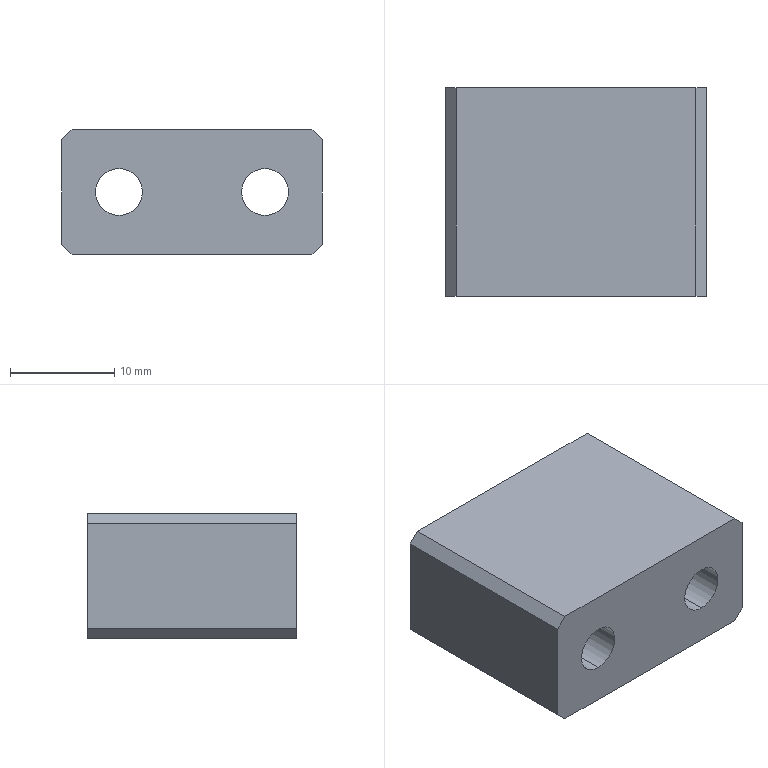Part | SolidWorks | features Chamfer 1, Extrusion 1, HoleWzd 1 | 1 solid | 20 faces | box 25 x 20 x 12 mm | volume 5021 mm3 | plane 12 | cylinder 8 | commonest cylinder face diameters 4.5 x4 8 x4
STEP:
#1=CARTESIAN_POINT('',(-7.,5.6,2.));
#2=VERTEX_POINT('',#1);
#3=CARTESIAN_POINT('',(-7.,5.6,10.));
#4=VERTEX_POINT('',#3);
#5=CARTESIAN_POINT('',(-7.,5.6,6.));
#6=DIRECTION('',(0.,1.,0.));
#7=DIRECTION('',(0.,0.,1.));
#8=AXIS2_PLACEMENT_3D('',#5,#6,#7);
#9=CIRCLE('',#8,4.);
#10=EDGE_CURVE('',#2,#4,#9,.T.);
#11=ORIENTED_EDGE('',*,*,#10,.F.);
#12=CARTESIAN_POINT('',(-7.,10.,2.));
#13=VERTEX_POINT('',#12);
#14=CARTESIAN_POINT('',(-7.,10.,2.));
#15=DIRECTION('',(0.,1.,0.));
#16=VECTOR('',#15,1000.);
#17=LINE('',#14,#16);
#18=EDGE_CURVE('',#2,#13,#17,.T.);
#19=ORIENTED_EDGE('',*,*,#18,.T.);
#20=CARTESIAN_POINT('',(-7.,10.,10.));
#21=VERTEX_POINT('',#20);
#22=CARTESIAN_POINT('',(-7.,10.,6.));
#23=DIRECTION('',(0.,1.,0.));
#24=DIRECTION('',(0.,0.,1.));
#25=AXIS2_PLACEMENT_3D('',#22,#23,#24);
#26=CIRCLE('',#25,4.);
#27=EDGE_CURVE('',#13,#21,#26,.T.);
#28=ORIENTED_EDGE('',*,*,#27,.T.);
#29=CARTESIAN_POINT('',(-7.,10.,10.));
#30=DIRECTION('',(0.,1.,0.));
#31=VECTOR('',#30,1000.);
#32=LINE('',#29,#31);
#33=EDGE_CURVE('',#4,#21,#32,.T.);
#34=ORIENTED_EDGE('',*,*,#33,.F.);
#35=EDGE_LOOP('',(#11,#19,#28,#34));
#36=FACE_OUTER_BOUND('',#35,.T.);
#37=CARTESIAN_POINT('',(-7.,10.,6.));
#38=DIRECTION('',(0.,1.,0.));
#39=DIRECTION('',(0.,0.,1.));
#40=AXIS2_PLACEMENT_3D('',#37,#38,#39);
#41=CYLINDRICAL_SURFACE('',#40,4.);
#42=ADVANCED_FACE('',(#36),#41,.F.);
#43=CARTESIAN_POINT('',(-7.,-10.,3.75));
#44=VERTEX_POINT('',#43);
#45=CARTESIAN_POINT('',(-7.,-10.,8.25));
#46=VERTEX_POINT('',#45);
#47=CARTESIAN_POINT('',(-7.,-10.,6.));
#48=DIRECTION('',(0.,1.,0.));
#49=DIRECTION('',(0.,0.,1.));
#50=AXIS2_PLACEMENT_3D('',#47,#48,#49);
#51=CIRCLE('',#50,2.25);
#52=EDGE_CURVE('',#44,#46,#51,.T.);
#53=ORIENTED_EDGE('',*,*,#52,.F.);
#54=CARTESIAN_POINT('',(-7.,5.6,3.75));
#55=VERTEX_POINT('',#54);
#56=CARTESIAN_POINT('',(-7.,10.,3.75));
#57=DIRECTION('',(0.,1.,0.));
#58=VECTOR('',#57,1000.);
#59=LINE('',#56,#58);
#60=EDGE_CURVE('',#44,#55,#59,.T.);
#61=ORIENTED_EDGE('',*,*,#60,.T.);
#62=CARTESIAN_POINT('',(-7.,5.6,8.25));
#63=VERTEX_POINT('',#62);
#64=CARTESIAN_POINT('',(-7.,5.6,6.));
#65=DIRECTION('',(0.,1.,0.));
#66=DIRECTION('',(0.,0.,1.));
#67=AXIS2_PLACEMENT_3D('',#64,#65,#66);
#68=CIRCLE('',#67,2.25);
#69=EDGE_CURVE('',#55,#63,#68,.T.);
#70=ORIENTED_EDGE('',*,*,#69,.T.);
#71=CARTESIAN_POINT('',(-7.,10.,8.25));
#72=DIRECTION('',(0.,1.,0.));
#73=VECTOR('',#72,1000.);
#74=LINE('',#71,#73);
#75=EDGE_CURVE('',#46,#63,#74,.T.);
#76=ORIENTED_EDGE('',*,*,#75,.F.);
#77=EDGE_LOOP('',(#53,#61,#70,#76));
#78=FACE_OUTER_BOUND('',#77,.T.);
#79=CARTESIAN_POINT('',(-7.,10.,6.));
#80=DIRECTION('',(0.,1.,0.));
#81=DIRECTION('',(0.,0.,1.));
#82=AXIS2_PLACEMENT_3D('',#79,#80,#81);
#83=CYLINDRICAL_SURFACE('',#82,2.25);
#84=ADVANCED_FACE('',(#78),#83,.F.);
#85=CARTESIAN_POINT('',(7.,5.6,2.));
#86=VERTEX_POINT('',#85);
#87=CARTESIAN_POINT('',(7.,5.6,10.));
#88=VERTEX_POINT('',#87);
#89=CARTESIAN_POINT('',(7.,5.6,6.));
#90=DIRECTION('',(0.,1.,0.));
#91=DIRECTION('',(0.,0.,1.));
#92=AXIS2_PLACEMENT_3D('',#89,#90,#91);
#93=CIRCLE('',#92,4.);
#94=EDGE_CURVE('',#86,#88,#93,.T.);
#95=ORIENTED_EDGE('',*,*,#94,.F.);
#96=CARTESIAN_POINT('',(7.,10.,2.));
#97=VERTEX_POINT('',#96);
#98=CARTESIAN_POINT('',(7.,10.,2.));
#99=DIRECTION('',(0.,1.,0.));
#100=VECTOR('',#99,1000.);
#101=LINE('',#98,#100);
#102=EDGE_CURVE('',#86,#97,#101,.T.);
#103=ORIENTED_EDGE('',*,*,#102,.T.);
#104=CARTESIAN_POINT('',(7.,10.,10.));
#105=VERTEX_POINT('',#104);
#106=CARTESIAN_POINT('',(7.,10.,6.));
#107=DIRECTION('',(0.,1.,0.));
#108=DIRECTION('',(0.,0.,1.));
#109=AXIS2_PLACEMENT_3D('',#106,#107,#108);
#110=CIRCLE('',#109,4.);
#111=EDGE_CURVE('',#97,#105,#110,.T.);
#112=ORIENTED_EDGE('',*,*,#111,.T.);
#113=CARTESIAN_POINT('',(7.,10.,10.));
#114=DIRECTION('',(0.,1.,0.));
#115=VECTOR('',#114,1000.);
#116=LINE('',#113,#115);
#117=EDGE_CURVE('',#88,#105,#116,.T.);
#118=ORIENTED_EDGE('',*,*,#117,.F.);
#119=EDGE_LOOP('',(#95,#103,#112,#118));
#120=FACE_OUTER_BOUND('',#119,.T.);
#121=CARTESIAN_POINT('',(7.,10.,6.));
#122=DIRECTION('',(0.,1.,0.));
#123=DIRECTION('',(0.,0.,1.));
#124=AXIS2_PLACEMENT_3D('',#121,#122,#123);
#125=CYLINDRICAL_SURFACE('',#124,4.);
#126=ADVANCED_FACE('',(#120),#125,.F.);
#127=CARTESIAN_POINT('',(7.,-10.,3.75));
#128=VERTEX_POINT('',#127);
#129=CARTESIAN_POINT('',(7.,-10.,8.25));
#130=VERTEX_POINT('',#129);
#131=CARTESIAN_POINT('',(7.,-10.,6.));
#132=DIRECTION('',(0.,1.,0.));
#133=DIRECTION('',(0.,0.,1.));
#134=AXIS2_PLACEMENT_3D('',#131,#132,#133);
#135=CIRCLE('',#134,2.25);
#136=EDGE_CURVE('',#128,#130,#135,.T.);
#137=ORIENTED_EDGE('',*,*,#136,.F.);
#138=CARTESIAN_POINT('',(7.,5.6,3.75));
#139=VERTEX_POINT('',#138);
#140=CARTESIAN_POINT('',(7.,10.,3.75));
#141=DIRECTION('',(0.,1.,0.));
#142=VECTOR('',#141,1000.);
#143=LINE('',#140,#142);
#144=EDGE_CURVE('',#128,#139,#143,.T.);
#145=ORIENTED_EDGE('',*,*,#144,.T.);
#146=CARTESIAN_POINT('',(7.,5.6,8.25));
#147=VERTEX_POINT('',#146);
#148=CARTESIAN_POINT('',(7.,5.6,6.));
#149=DIRECTION('',(0.,1.,0.));
#150=DIRECTION('',(0.,0.,1.));
#151=AXIS2_PLACEMENT_3D('',#148,#149,#150);
#152=CIRCLE('',#151,2.25);
#153=EDGE_CURVE('',#139,#147,#152,.T.);
#154=ORIENTED_EDGE('',*,*,#153,.T.);
#155=CARTESIAN_POINT('',(7.,10.,8.25));
#156=DIRECTION('',(0.,1.,0.));
#157=VECTOR('',#156,1000.);
#158=LINE('',#155,#157);
#159=EDGE_CURVE('',#130,#147,#158,.T.);
#160=ORIENTED_EDGE('',*,*,#159,.F.);
#161=EDGE_LOOP('',(#137,#145,#154,#160));
#162=FACE_OUTER_BOUND('',#161,.T.);
#163=CARTESIAN_POINT('',(7.,10.,6.));
#164=DIRECTION('',(0.,1.,0.));
#165=DIRECTION('',(0.,0.,1.));
#166=AXIS2_PLACEMENT_3D('',#163,#164,#165);
#167=CYLINDRICAL_SURFACE('',#166,2.25);
#168=ADVANCED_FACE('',(#162),#167,.F.);
#169=CARTESIAN_POINT('',(12.5,-10.,11.));
#170=VERTEX_POINT('',#169);
#171=CARTESIAN_POINT('',(12.5,-10.,1.));
#172=VERTEX_POINT('',#171);
#173=CARTESIAN_POINT('',(12.5,-10.,12.));
#174=DIRECTION('',(0.,0.,-1.));
#175=VECTOR('',#174,1000.);
#176=LINE('',#173,#175);
#177=EDGE_CURVE('',#170,#172,#176,.T.);
#178=ORIENTED_EDGE('',*,*,#177,.T.);
#179=CARTESIAN_POINT('',(12.5,10.,1.));
#180=VERTEX_POINT('',#179);
#181=CARTESIAN_POINT('',(12.5,10.,1.));
#182=DIRECTION('',(0.,1.,0.));
#183=VECTOR('',#182,1000.);
#184=LINE('',#181,#183);
#185=EDGE_CURVE('',#172,#180,#184,.T.);
#186=ORIENTED_EDGE('',*,*,#185,.T.);
#187=CARTESIAN_POINT('',(12.5,10.,11.));
#188=VERTEX_POINT('',#187);
#189=CARTESIAN_POINT('',(12.5,10.,12.));
#190=DIRECTION('',(0.,0.,-1.));
#191=VECTOR('',#190,1000.);
#192=LINE('',#189,#191);
#193=EDGE_CURVE('',#188,#180,#192,.T.);
#194=ORIENTED_EDGE('',*,*,#193,.F.);
#195=CARTESIAN_POINT('',(12.5,-10.,11.));
#196=DIRECTION('',(0.,-1.,0.));
#197=VECTOR('',#196,1000.);
#198=LINE('',#195,#197);
#199=EDGE_CURVE('',#188,#170,#198,.T.);
#200=ORIENTED_EDGE('',*,*,#199,.T.);
#201=EDGE_LOOP('',(#178,#186,#194,#200));
#202=FACE_OUTER_BOUND('',#201,.T.);
#203=CARTESIAN_POINT('',(12.5,10.,12.));
#204=DIRECTION('',(-1.,0.,0.));
#205=DIRECTION('',(0.,-1.,0.));
#206=AXIS2_PLACEMENT_3D('',#203,#204,#205);
#207=PLANE('',#206);
#208=ADVANCED_FACE('',(#202),#207,.F.);
#209=CARTESIAN_POINT('',(-7.,10.,6.));
#210=DIRECTION('',(0.,1.,0.));
#211=DIRECTION('',(0.,0.,1.));
#212=AXIS2_PLACEMENT_3D('',#209,#210,#211);
#213=CIRCLE('',#212,4.);
#214=EDGE_CURVE('',#21,#13,#213,.T.);
#215=ORIENTED_EDGE('',*,*,#214,.F.);
#216=ORIENTED_EDGE('',*,*,#27,.F.);
#217=EDGE_LOOP('',(#215,#216));
#218=FACE_BOUND('',#217,.T.);
#219=CARTESIAN_POINT('',(7.,10.,6.));
#220=DIRECTION('',(0.,1.,0.));
#221=DIRECTION('',(0.,0.,1.));
#222=AXIS2_PLACEMENT_3D('',#219,#220,#221);
#223=CIRCLE('',#222,4.);
#224=EDGE_CURVE('',#105,#97,#223,.T.);
#225=ORIENTED_EDGE('',*,*,#224,.F.);
#226=ORIENTED_EDGE('',*,*,#111,.F.);
#227=EDGE_LOOP('',(#225,#226));
#228=FACE_BOUND('',#227,.T.);
#229=CARTESIAN_POINT('',(11.5,10.,0.));
#230=VERTEX_POINT('',#229);
#231=CARTESIAN_POINT('',(-11.5,10.,0.));
#232=VERTEX_POINT('',#231);
#233=CARTESIAN_POINT('',(-12.5,10.,0.));
#234=DIRECTION('',(-1.,0.,0.));
#235=VECTOR('',#234,1000.);
#236=LINE('',#233,#235);
#237=EDGE_CURVE('',#230,#232,#236,.T.);
#238=ORIENTED_EDGE('',*,*,#237,.T.);
#239=CARTESIAN_POINT('',(-12.5,10.,1.));
#240=VERTEX_POINT('',#239);
#241=CARTESIAN_POINT('',(-12.5,10.,1.));
#242=DIRECTION('',(-0.7071,0.,0.7071));
#243=VECTOR('',#242,1000.);
#244=LINE('',#241,#243);
#245=EDGE_CURVE('',#232,#240,#244,.T.);
#246=ORIENTED_EDGE('',*,*,#245,.T.);
#247=CARTESIAN_POINT('',(-12.5,10.,11.));
#248=VERTEX_POINT('',#247);
#249=CARTESIAN_POINT('',(-12.5,10.,12.));
#250=DIRECTION('',(0.,0.,-1.));
#251=VECTOR('',#250,1000.);
#252=LINE('',#249,#251);
#253=EDGE_CURVE('',#248,#240,#252,.T.);
#254=ORIENTED_EDGE('',*,*,#253,.F.);
#255=CARTESIAN_POINT('',(-11.5,10.,12.));
#256=VERTEX_POINT('',#255);
#257=CARTESIAN_POINT('',(-11.5,10.,12.));
#258=DIRECTION('',(0.7071,0.,0.7071));
#259=VECTOR('',#258,1000.);
#260=LINE('',#257,#259);
#261=EDGE_CURVE('',#248,#256,#260,.T.);
#262=ORIENTED_EDGE('',*,*,#261,.T.);
#263=CARTESIAN_POINT('',(11.5,10.,12.));
#264=VERTEX_POINT('',#263);
#265=CARTESIAN_POINT('',(-12.5,10.,12.));
#266=DIRECTION('',(-1.,0.,0.));
#267=VECTOR('',#266,1000.);
#268=LINE('',#265,#267);
#269=EDGE_CURVE('',#264,#256,#268,.T.);
#270=ORIENTED_EDGE('',*,*,#269,.F.);
#271=CARTESIAN_POINT('',(11.5,10.,12.));
#272=DIRECTION('',(0.7071,0.,-0.7071));
#273=VECTOR('',#272,1000.);
#274=LINE('',#271,#273);
#275=EDGE_CURVE('',#264,#188,#274,.T.);
#276=ORIENTED_EDGE('',*,*,#275,.T.);
#277=ORIENTED_EDGE('',*,*,#193,.T.);
#278=CARTESIAN_POINT('',(12.5,10.,1.));
#279=DIRECTION('',(-0.7071,0.,-0.7071));
#280=VECTOR('',#279,1000.);
#281=LINE('',#278,#280);
#282=EDGE_CURVE('',#180,#230,#281,.T.);
#283=ORIENTED_EDGE('',*,*,#282,.T.);
#284=EDGE_LOOP('',(#238,#246,#254,#262,#270,#276,#277,#283));
#285=FACE_OUTER_BOUND('',#284,.T.);
#286=CARTESIAN_POINT('',(-12.5,10.,12.));
#287=DIRECTION('',(0.,-1.,0.));
#288=DIRECTION('',(0.,0.,-1.));
#289=AXIS2_PLACEMENT_3D('',#286,#287,#288);
#290=PLANE('',#289);
#291=ADVANCED_FACE('',(#218,#228,#285),#290,.F.);
#292=ORIENTED_EDGE('',*,*,#253,.T.);
#293=CARTESIAN_POINT('',(-12.5,-10.,1.));
#294=VERTEX_POINT('',#293);
#295=CARTESIAN_POINT('',(-12.5,10.,1.));
#296=DIRECTION('',(0.,-1.,0.));
#297=VECTOR('',#296,1000.);
#298=LINE('',#295,#297);
#299=EDGE_CURVE('',#240,#294,#298,.T.);
#300=ORIENTED_EDGE('',*,*,#299,.T.);
#301=CARTESIAN_POINT('',(-12.5,-10.,11.));
#302=VERTEX_POINT('',#301);
#303=CARTESIAN_POINT('',(-12.5,-10.,12.));
#304=DIRECTION('',(0.,0.,-1.));
#305=VECTOR('',#304,1000.);
#306=LINE('',#303,#305);
#307=EDGE_CURVE('',#302,#294,#306,.T.);
#308=ORIENTED_EDGE('',*,*,#307,.F.);
#309=CARTESIAN_POINT('',(-12.5,10.,11.));
#310=DIRECTION('',(0.,1.,0.));
#311=VECTOR('',#310,1000.);
#312=LINE('',#309,#311);
#313=EDGE_CURVE('',#302,#248,#312,.T.);
#314=ORIENTED_EDGE('',*,*,#313,.T.);
#315=EDGE_LOOP('',(#292,#300,#308,#314));
#316=FACE_OUTER_BOUND('',#315,.T.);
#317=CARTESIAN_POINT('',(-12.5,10.,12.));
#318=DIRECTION('',(1.,0.,0.));
#319=DIRECTION('',(0.,1.,0.));
#320=AXIS2_PLACEMENT_3D('',#317,#318,#319);
#321=PLANE('',#320);
#322=ADVANCED_FACE('',(#316),#321,.F.);
#323=CARTESIAN_POINT('',(-7.,-10.,6.));
#324=DIRECTION('',(0.,1.,0.));
#325=DIRECTION('',(0.,0.,1.));
#326=AXIS2_PLACEMENT_3D('',#323,#324,#325);
#327=CIRCLE('',#326,2.25);
#328=EDGE_CURVE('',#46,#44,#327,.T.);
#329=ORIENTED_EDGE('',*,*,#328,.T.);
#330=ORIENTED_EDGE('',*,*,#52,.T.);
#331=EDGE_LOOP('',(#329,#330));
#332=FACE_BOUND('',#331,.T.);
#333=CARTESIAN_POINT('',(7.,-10.,6.));
#334=DIRECTION('',(0.,1.,0.));
#335=DIRECTION('',(0.,0.,1.));
#336=AXIS2_PLACEMENT_3D('',#333,#334,#335);
#337=CIRCLE('',#336,2.25);
#338=EDGE_CURVE('',#130,#128,#337,.T.);
#339=ORIENTED_EDGE('',*,*,#338,.T.);
#340=ORIENTED_EDGE('',*,*,#136,.T.);
#341=EDGE_LOOP('',(#339,#340));
#342=FACE_BOUND('',#341,.T.);
#343=ORIENTED_EDGE('',*,*,#307,.T.);
#344=CARTESIAN_POINT('',(-11.5,-10.,0.));
#345=VERTEX_POINT('',#344);
#346=CARTESIAN_POINT('',(-12.5,-10.,1.));
#347=DIRECTION('',(0.7071,0.,-0.7071));
#348=VECTOR('',#347,1000.);
#349=LINE('',#346,#348);
#350=EDGE_CURVE('',#294,#345,#349,.T.);
#351=ORIENTED_EDGE('',*,*,#350,.T.);
#352=CARTESIAN_POINT('',(11.5,-10.,0.));
#353=VERTEX_POINT('',#352);
#354=CARTESIAN_POINT('',(-12.5,-10.,0.));
#355=DIRECTION('',(1.,0.,0.));
#356=VECTOR('',#355,1000.);
#357=LINE('',#354,#356);
#358=EDGE_CURVE('',#345,#353,#357,.T.);
#359=ORIENTED_EDGE('',*,*,#358,.T.);
#360=CARTESIAN_POINT('',(12.5,-10.,1.));
#361=DIRECTION('',(0.7071,0.,0.7071));
#362=VECTOR('',#361,1000.);
#363=LINE('',#360,#362);
#364=EDGE_CURVE('',#353,#172,#363,.T.);
#365=ORIENTED_EDGE('',*,*,#364,.T.);
#366=ORIENTED_EDGE('',*,*,#177,.F.);
#367=CARTESIAN_POINT('',(11.5,-10.,12.));
#368=VERTEX_POINT('',#367);
#369=CARTESIAN_POINT('',(11.5,-10.,12.));
#370=DIRECTION('',(-0.7071,0.,0.7071));
#371=VECTOR('',#370,1000.);
#372=LINE('',#369,#371);
#373=EDGE_CURVE('',#170,#368,#372,.T.);
#374=ORIENTED_EDGE('',*,*,#373,.T.);
#375=CARTESIAN_POINT('',(-11.5,-10.,12.));
#376=VERTEX_POINT('',#375);
#377=CARTESIAN_POINT('',(-12.5,-10.,12.));
#378=DIRECTION('',(1.,0.,0.));
#379=VECTOR('',#378,1000.);
#380=LINE('',#377,#379);
#381=EDGE_CURVE('',#376,#368,#380,.T.);
#382=ORIENTED_EDGE('',*,*,#381,.F.);
#383=CARTESIAN_POINT('',(-11.5,-10.,12.));
#384=DIRECTION('',(-0.7071,0.,-0.7071));
#385=VECTOR('',#384,1000.);
#386=LINE('',#383,#385);
#387=EDGE_CURVE('',#376,#302,#386,.T.);
#388=ORIENTED_EDGE('',*,*,#387,.T.);
#389=EDGE_LOOP('',(#343,#351,#359,#365,#366,#374,#382,#388));
#390=FACE_OUTER_BOUND('',#389,.T.);
#391=CARTESIAN_POINT('',(-12.5,-10.,12.));
#392=DIRECTION('',(0.,1.,0.));
#393=DIRECTION('',(0.,0.,1.));
#394=AXIS2_PLACEMENT_3D('',#391,#392,#393);
#395=PLANE('',#394);
#396=ADVANCED_FACE('',(#332,#342,#390),#395,.F.);
#397=ORIENTED_EDGE('',*,*,#381,.T.);
#398=CARTESIAN_POINT('',(11.5,10.,12.));
#399=DIRECTION('',(0.,1.,0.));
#400=VECTOR('',#399,1000.);
#401=LINE('',#398,#400);
#402=EDGE_CURVE('',#368,#264,#401,.T.);
#403=ORIENTED_EDGE('',*,*,#402,.T.);
#404=ORIENTED_EDGE('',*,*,#269,.T.);
#405=CARTESIAN_POINT('',(-11.5,-10.,12.));
#406=DIRECTION('',(0.,-1.,0.));
#407=VECTOR('',#406,1000.);
#408=LINE('',#405,#407);
#409=EDGE_CURVE('',#256,#376,#408,.T.);
#410=ORIENTED_EDGE('',*,*,#409,.T.);
#411=EDGE_LOOP('',(#397,#403,#404,#410));
#412=FACE_OUTER_BOUND('',#411,.T.);
#413=CARTESIAN_POINT('',(0.,0.,12.));
#414=DIRECTION('',(0.,0.,1.));
#415=DIRECTION('',(1.,0.,0.));
#416=AXIS2_PLACEMENT_3D('',#413,#414,#415);
#417=PLANE('',#416);
#418=ADVANCED_FACE('',(#412),#417,.T.);
#419=ORIENTED_EDGE('',*,*,#358,.F.);
#420=CARTESIAN_POINT('',(-11.5,0.,0.));
#421=DIRECTION('',(0.,1.,0.));
#422=VECTOR('',#421,1000.);
#423=LINE('',#420,#422);
#424=EDGE_CURVE('',#345,#232,#423,.T.);
#425=ORIENTED_EDGE('',*,*,#424,.T.);
#426=ORIENTED_EDGE('',*,*,#237,.F.);
#427=CARTESIAN_POINT('',(11.5,0.,0.));
#428=DIRECTION('',(0.,-1.,0.));
#429=VECTOR('',#428,1000.);
#430=LINE('',#427,#429);
#431=EDGE_CURVE('',#230,#353,#430,.T.);
#432=ORIENTED_EDGE('',*,*,#431,.T.);
#433=EDGE_LOOP('',(#419,#425,#426,#432));
#434=FACE_OUTER_BOUND('',#433,.T.);
#435=CARTESIAN_POINT('',(0.,0.,0.));
#436=DIRECTION('',(0.,0.,1.));
#437=DIRECTION('',(1.,0.,0.));
#438=AXIS2_PLACEMENT_3D('',#435,#436,#437);
#439=PLANE('',#438);
#440=ADVANCED_FACE('',(#434),#439,.F.);
#441=ORIENTED_EDGE('',*,*,#144,.F.);
#442=ORIENTED_EDGE('',*,*,#338,.F.);
#443=ORIENTED_EDGE('',*,*,#159,.T.);
#444=CARTESIAN_POINT('',(7.,5.6,6.));
#445=DIRECTION('',(0.,1.,0.));
#446=DIRECTION('',(0.,0.,1.));
#447=AXIS2_PLACEMENT_3D('',#444,#445,#446);
#448=CIRCLE('',#447,2.25);
#449=EDGE_CURVE('',#147,#139,#448,.T.);
#450=ORIENTED_EDGE('',*,*,#449,.T.);
#451=EDGE_LOOP('',(#441,#442,#443,#450));
#452=FACE_OUTER_BOUND('',#451,.T.);
#453=CARTESIAN_POINT('',(7.,10.,6.));
#454=DIRECTION('',(0.,1.,0.));
#455=DIRECTION('',(0.,0.,1.));
#456=AXIS2_PLACEMENT_3D('',#453,#454,#455);
#457=CYLINDRICAL_SURFACE('',#456,2.25);
#458=ADVANCED_FACE('',(#452),#457,.F.);
#459=ORIENTED_EDGE('',*,*,#449,.F.);
#460=ORIENTED_EDGE('',*,*,#153,.F.);
#461=EDGE_LOOP('',(#459,#460));
#462=FACE_BOUND('',#461,.T.);
#463=CARTESIAN_POINT('',(7.,5.6,6.));
#464=DIRECTION('',(0.,1.,0.));
#465=DIRECTION('',(0.,0.,1.));
#466=AXIS2_PLACEMENT_3D('',#463,#464,#465);
#467=CIRCLE('',#466,4.);
#468=EDGE_CURVE('',#88,#86,#467,.T.);
#469=ORIENTED_EDGE('',*,*,#468,.T.);
#470=ORIENTED_EDGE('',*,*,#94,.T.);
#471=EDGE_LOOP('',(#469,#470));
#472=FACE_OUTER_BOUND('',#471,.T.);
#473=CARTESIAN_POINT('',(9.25,5.6,6.));
#474=DIRECTION('',(0.,-1.,0.));
#475=DIRECTION('',(0.,0.,-1.));
#476=AXIS2_PLACEMENT_3D('',#473,#474,#475);
#477=PLANE('',#476);
#478=ADVANCED_FACE('',(#462,#472),#477,.F.);
#479=ORIENTED_EDGE('',*,*,#102,.F.);
#480=ORIENTED_EDGE('',*,*,#468,.F.);
#481=ORIENTED_EDGE('',*,*,#117,.T.);
#482=ORIENTED_EDGE('',*,*,#224,.T.);
#483=EDGE_LOOP('',(#479,#480,#481,#482));
#484=FACE_OUTER_BOUND('',#483,.T.);
#485=CARTESIAN_POINT('',(7.,10.,6.));
#486=DIRECTION('',(0.,1.,0.));
#487=DIRECTION('',(0.,0.,1.));
#488=AXIS2_PLACEMENT_3D('',#485,#486,#487);
#489=CYLINDRICAL_SURFACE('',#488,4.);
#490=ADVANCED_FACE('',(#484),#489,.F.);
#491=ORIENTED_EDGE('',*,*,#60,.F.);
#492=ORIENTED_EDGE('',*,*,#328,.F.);
#493=ORIENTED_EDGE('',*,*,#75,.T.);
#494=CARTESIAN_POINT('',(-7.,5.6,6.));
#495=DIRECTION('',(0.,1.,0.));
#496=DIRECTION('',(0.,0.,1.));
#497=AXIS2_PLACEMENT_3D('',#494,#495,#496);
#498=CIRCLE('',#497,2.25);
#499=EDGE_CURVE('',#63,#55,#498,.T.);
#500=ORIENTED_EDGE('',*,*,#499,.T.);
#501=EDGE_LOOP('',(#491,#492,#493,#500));
#502=FACE_OUTER_BOUND('',#501,.T.);
#503=CARTESIAN_POINT('',(-7.,10.,6.));
#504=DIRECTION('',(0.,1.,0.));
#505=DIRECTION('',(0.,0.,1.));
#506=AXIS2_PLACEMENT_3D('',#503,#504,#505);
#507=CYLINDRICAL_SURFACE('',#506,2.25);
#508=ADVANCED_FACE('',(#502),#507,.F.);
#509=ORIENTED_EDGE('',*,*,#499,.F.);
#510=ORIENTED_EDGE('',*,*,#69,.F.);
#511=EDGE_LOOP('',(#509,#510));
#512=FACE_BOUND('',#511,.T.);
#513=CARTESIAN_POINT('',(-7.,5.6,6.));
#514=DIRECTION('',(0.,1.,0.));
#515=DIRECTION('',(0.,0.,1.));
#516=AXIS2_PLACEMENT_3D('',#513,#514,#515);
#517=CIRCLE('',#516,4.);
#518=EDGE_CURVE('',#4,#2,#517,.T.);
#519=ORIENTED_EDGE('',*,*,#518,.T.);
#520=ORIENTED_EDGE('',*,*,#10,.T.);
#521=EDGE_LOOP('',(#519,#520));
#522=FACE_OUTER_BOUND('',#521,.T.);
#523=CARTESIAN_POINT('',(-4.75,5.6,6.));
#524=DIRECTION('',(0.,-1.,0.));
#525=DIRECTION('',(0.,0.,-1.));
#526=AXIS2_PLACEMENT_3D('',#523,#524,#525);
#527=PLANE('',#526);
#528=ADVANCED_FACE('',(#512,#522),#527,.F.);
#529=ORIENTED_EDGE('',*,*,#18,.F.);
#530=ORIENTED_EDGE('',*,*,#518,.F.);
#531=ORIENTED_EDGE('',*,*,#33,.T.);
#532=ORIENTED_EDGE('',*,*,#214,.T.);
#533=EDGE_LOOP('',(#529,#530,#531,#532));
#534=FACE_OUTER_BOUND('',#533,.T.);
#535=CARTESIAN_POINT('',(-7.,10.,6.));
#536=DIRECTION('',(0.,1.,0.));
#537=DIRECTION('',(0.,0.,1.));
#538=AXIS2_PLACEMENT_3D('',#535,#536,#537);
#539=CYLINDRICAL_SURFACE('',#538,4.);
#540=ADVANCED_FACE('',(#534),#539,.F.);
#541=ORIENTED_EDGE('',*,*,#245,.F.);
#542=ORIENTED_EDGE('',*,*,#424,.F.);
#543=ORIENTED_EDGE('',*,*,#350,.F.);
#544=ORIENTED_EDGE('',*,*,#299,.F.);
#545=EDGE_LOOP('',(#541,#542,#543,#544));
#546=FACE_OUTER_BOUND('',#545,.T.);
#547=CARTESIAN_POINT('',(-12.5,10.,1.));
#548=DIRECTION('',(0.7071,0.,0.7071));
#549=DIRECTION('',(0.,-1.,0.));
#550=AXIS2_PLACEMENT_3D('',#547,#548,#549);
#551=PLANE('',#550);
#552=ADVANCED_FACE('',(#546),#551,.F.);
#553=ORIENTED_EDGE('',*,*,#364,.F.);
#554=ORIENTED_EDGE('',*,*,#431,.F.);
#555=ORIENTED_EDGE('',*,*,#282,.F.);
#556=ORIENTED_EDGE('',*,*,#185,.F.);
#557=EDGE_LOOP('',(#553,#554,#555,#556));
#558=FACE_OUTER_BOUND('',#557,.T.);
#559=CARTESIAN_POINT('',(12.5,10.,1.));
#560=DIRECTION('',(-0.7071,0.,0.7071));
#561=DIRECTION('',(0.,1.,0.));
#562=AXIS2_PLACEMENT_3D('',#559,#560,#561);
#563=PLANE('',#562);
#564=ADVANCED_FACE('',(#558),#563,.F.);
#565=ORIENTED_EDGE('',*,*,#373,.F.);
#566=ORIENTED_EDGE('',*,*,#199,.F.);
#567=ORIENTED_EDGE('',*,*,#275,.F.);
#568=ORIENTED_EDGE('',*,*,#402,.F.);
#569=EDGE_LOOP('',(#565,#566,#567,#568));
#570=FACE_OUTER_BOUND('',#569,.T.);
#571=CARTESIAN_POINT('',(11.5,0.,12.));
#572=DIRECTION('',(0.7071,0.,0.7071));
#573=DIRECTION('',(0.,-1.,0.));
#574=AXIS2_PLACEMENT_3D('',#571,#572,#573);
#575=PLANE('',#574);
#576=ADVANCED_FACE('',(#570),#575,.T.);
#577=ORIENTED_EDGE('',*,*,#261,.F.);
#578=ORIENTED_EDGE('',*,*,#313,.F.);
#579=ORIENTED_EDGE('',*,*,#387,.F.);
#580=ORIENTED_EDGE('',*,*,#409,.F.);
#581=EDGE_LOOP('',(#577,#578,#579,#580));
#582=FACE_OUTER_BOUND('',#581,.T.);
#583=CARTESIAN_POINT('',(-11.5,0.,12.));
#584=DIRECTION('',(-0.7071,0.,0.7071));
#585=DIRECTION('',(0.,1.,0.));
#586=AXIS2_PLACEMENT_3D('',#583,#584,#585);
#587=PLANE('',#586);
#588=ADVANCED_FACE('',(#582),#587,.T.);
#589=CLOSED_SHELL('',(#42,#84,#126,#168,#208,#291,#322,#396,#418,#440,#458,#478,#490,#508,#528,#540,#552,#564,#576,#588));
#590=MANIFOLD_SOLID_BREP('',#589);
#591=CARTESIAN_POINT('',(0.,0.,0.));
#592=DIRECTION('',(0.,0.,1.));
#593=DIRECTION('',(1.,0.,0.));
#594=AXIS2_PLACEMENT_3D('',#591,#592,#593);
#595=(LENGTH_UNIT()NAMED_UNIT(*)SI_UNIT(.MILLI.,.METRE.));
#596=UNCERTAINTY_MEASURE_WITH_UNIT(LENGTH_MEASURE(0.00001),#595,'','');
#597=(NAMED_UNIT(*)PLANE_ANGLE_UNIT()SI_UNIT($,.RADIAN.));
#598=(NAMED_UNIT(*)SI_UNIT($,.STERADIAN.)SOLID_ANGLE_UNIT());
#599=(GEOMETRIC_REPRESENTATION_CONTEXT(3)GLOBAL_UNCERTAINTY_ASSIGNED_CONTEXT((#596))GLOBAL_UNIT_ASSIGNED_CONTEXT((#595,#597,#598))REPRESENTATION_CONTEXT('',''));
#600=ADVANCED_BREP_SHAPE_REPRESENTATION('',(#590,#594),#599);